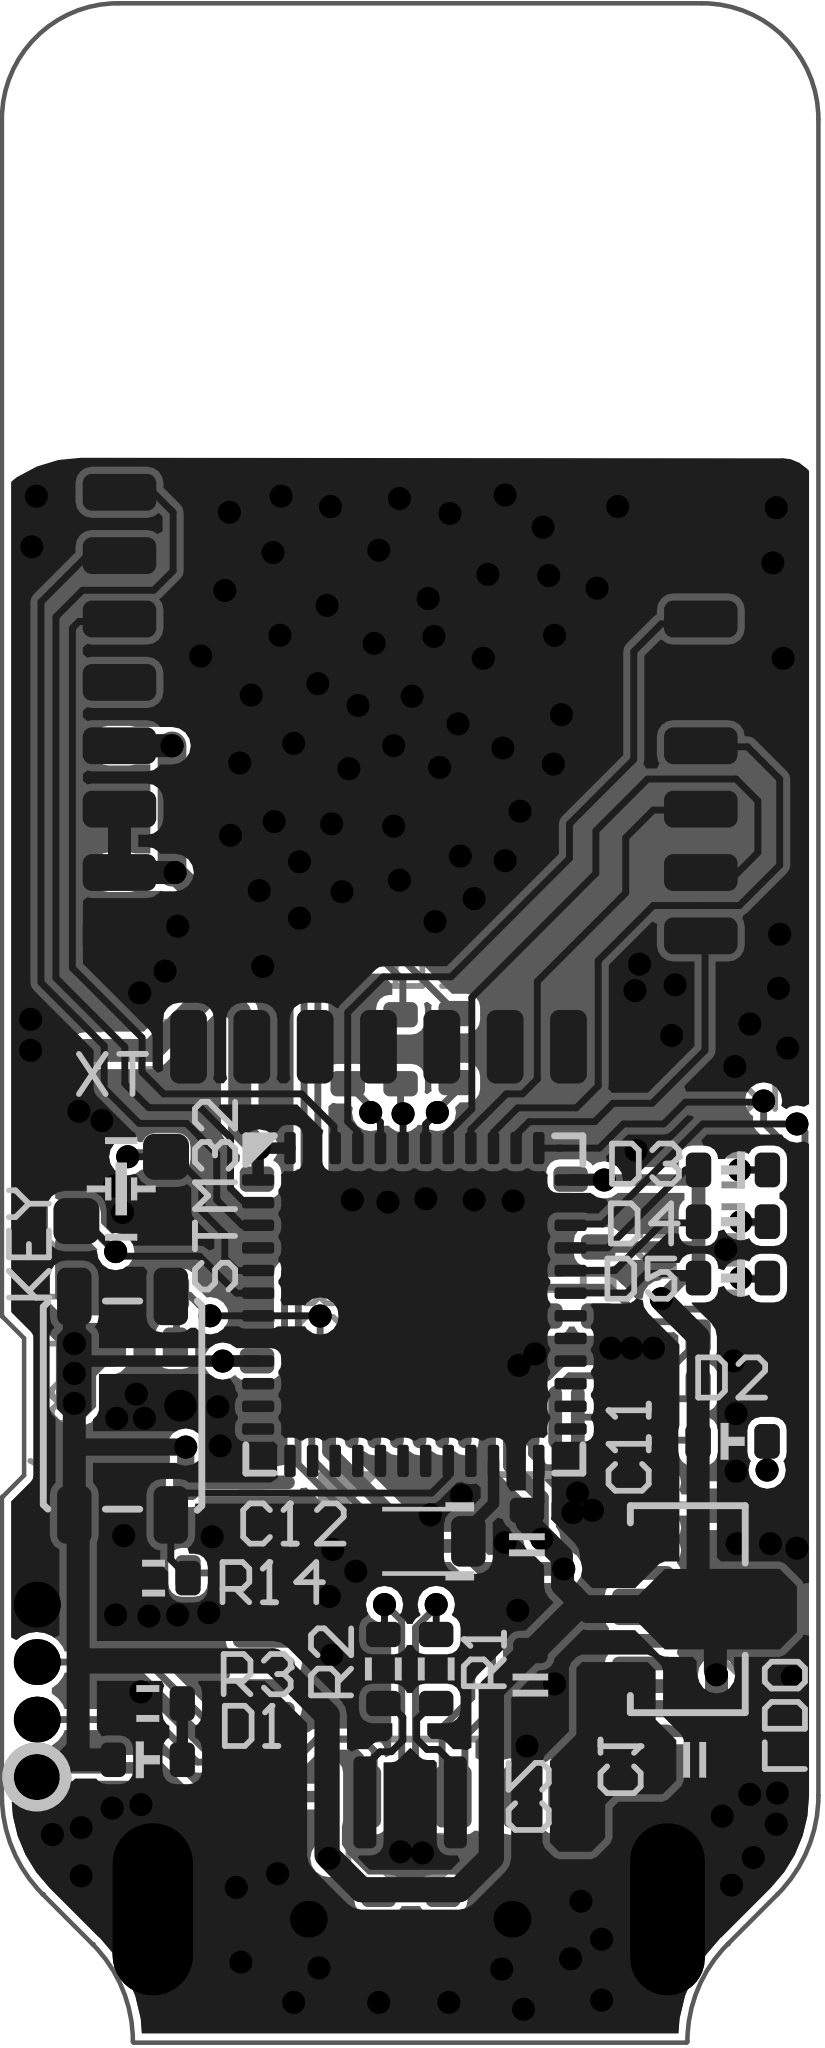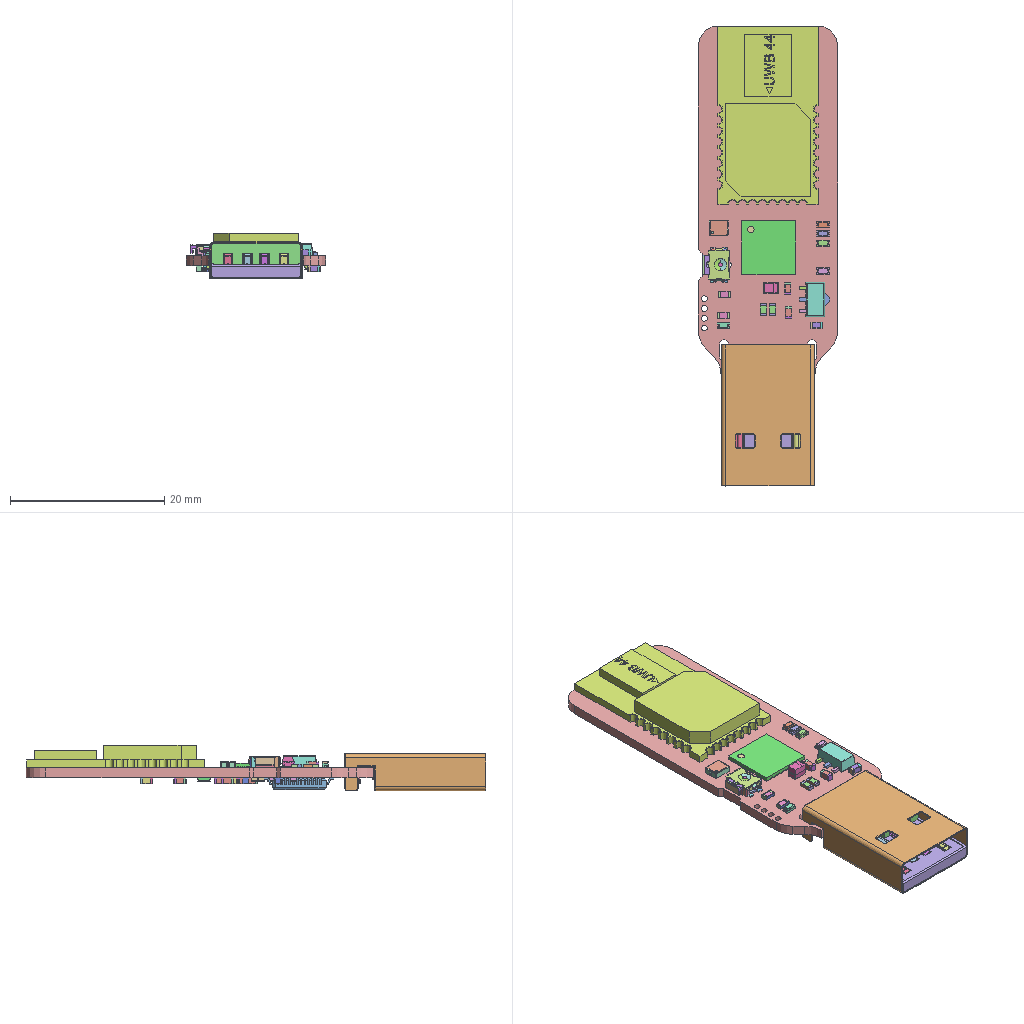Circuit board layout | Altium Designer | box 18.1 x 59.7 x 5.9 mm
Layer stack:
# Altium Designer layer stack of 9 (unit mm; dielectric type: 0 none, 1 core, 2 prepreg, 3 surface material)
index,name,kind,layer,copper_thickness_mm,dielectric_type,dielectric_thickness_mm,dielectric_material,dielectric_constant
0,Top Paste,other,,,,,,
1,Top Overlay,other,,,,,,
2,Top Solder,dielectric,,,3,0.01,Solder Resist,3.5
3,Top Layer,copper,Top Layer,0.03,,,,
4,Dielectric1,dielectric,,,1,1.2,,4.2
5,Bottom Layer,copper,Bottom Layer,0.03,,,,
6,Bottom Solder,dielectric,,,3,0.01,Solder Resist,3.5
7,Bottom Overlay,other,,,,,,
8,Bottom Paste,other,,,,,,
# drill layer pairs: low layer,high layer
drill_pair,Top Layer,Bottom Layer
Part placement:
Designator,Comment,Layer,Footprint,Center-X(mm),Center-Y(mm),Rotation
LDO,AMS1117,TopLayer,SOT89-3,10.617,9.55,360
USB,USB_Plug_TypeA,TopLayer,USB_Plug_TypeA,6.104,3.992,270
XT,XTAL_2520_4P,TopLayer,XT_2520_4,-0.2837,18.834,360
R14,Res_0603,TopLayer,RES_0603,0.4318,10.236,360
R13,Res_0603,BottomLayer,RES_0603,0.1524,15.392,180
R12,Res_0603,BottomLayer,RES_0603,4.724,21.92,90
R11,Res_0603,BottomLayer,RES_0603,7.112,21.946,90
R10,Res_0603,BottomLayer,RES_0603,5.893,21.92,90
R9,Res_0603,BottomLayer,RES_0603,13.614,11.836,180
R8,Res_0603,BottomLayer,RES_0603,13.233,14.453,180
R7,Res_0603,BottomLayer,RES_0603,13.233,15.57,180
R6,Res_0603,BottomLayer,RES_0603,0.4318,10.363,360
R5,Res_0603,BottomLayer,RES_0603,10.262,16.789,90
R4,Res_0603,BottomLayer,RES_0603,13.233,13.259,360
R3,Res_0603,TopLayer,RES_0603,0.3048,7.468,360
R2,Res_0603,TopLayer,RES_0603,5.512,8.23,90
R1,Res_0603,TopLayer,RES_0603,6.68,8.23,90
KEY,ButtonTACT,TopLayer,ButtonTACT_3.5*3.55_90,-0.1524,14.046,90
C17,Cap_0603,BottomLayer,CAP_0603,-0.3302,29.388,90
C16,Cap_0603,BottomLayer,CAP_0603,-0.3302,25.07,270
C13,Cap_0603,BottomLayer,CAP_0603,0.1778,16.535,360
C11,Cap_0603,TopLayer,CAP_0603,8.687,10.973,90
C10,Cap_0603,BottomLayer,CAP_0603,9.652,19.812,270
C9,Cap_0603,BottomLayer,CAP_0603,2.718,18.288,90
C8,Cap_0603,BottomLayer,CAP_0603,2.718,15.799,270
C7,Cap_0603,BottomLayer,CAP_0603,13.64,6.858,180
C6,Cap_0603,BottomLayer,CAP_0603,0.381,12.344,360
C5,Cap_0603,BottomLayer,CAP_0603,6.833,2.489,90
C4,Cap_0603,BottomLayer,CAP_0603,5.41,2.489,90
C3,Cap_0603,BottomLayer,CAP_0603,9.093,16.789,270
STM32,STM32F411C,TopLayer,QFN_P0.5_48,6.198,16.281,360
STM32J,STM32F072C,BottomLayer,LQFP_P0.5_48,7.061,9.601,270
DWM,DWM1000,TopLayer,DWM1000,6.104,28.099,0
D2,LED_0603,TopLayer,LED_0603_ORANGE,13.233,13.259,360
D1,LED_0603,TopLayer,LED_0603_YELLOW,0.3048,6.223,360
C1,Cap_0603,TopLayer,CAP_0603,12.395,6.223,180
C2,Cap_0603,TopLayer,CAP_0603,8.763,7.874,90
D3,LED_0603,TopLayer,LED_0603_RED,13.242,19.253,180
D4,LED_0603,TopLayer,LED_0603_GREEN,13.242,18.11,180
D5,LED_0603,TopLayer,LED_0603_BLUE,13.242,16.866,180
R15,Res_0603,BottomLayer,RES_0603,13.242,19.253,180
R16,Res_0603,BottomLayer,RES_0603,13.242,18.11,180
R17,Res_0603,BottomLayer,RES_0603,13.242,16.866,180
C12,Cap_Tan_0805,TopLayer,CAP_TAN_P0805,6.502,11.049,180
C15,Cap_0603,BottomLayer,CAP_0603,-1.27,18.923,270
C14,Cap_0603,BottomLayer,CAP_0603,0.7112,18.872,90
Pad and via stacks:
# Altium Designer via and pad stacks of 9 (unit mm). Each distinct definition once, with the count of objects using it.
# via: kind,start_layer,end_layer,hole_mm,diameter_mm,mode(0 simple;1 top-mid-bottom;2 full stack),diameter_per_layer,count,example_net
# pad: kind,layer,hole_mm,hole_type(0 round;1 square;2 slot),plating,top_size,top_shape(1 round;2 rect;3 octagon;9 rounded rect),mid_size,bottom_size,mode,footprint,size_per_layer,count,example
pad,Top Layer,0,0,plated,0.762x0.5588,9,0.762x0.5588,0.762x0.5588,0,RES_0603,,8,R3.2
pad,Top Layer,0,0,plated,1.118x0.762,9,1.118x0.762,1.118x0.762,0,CAP_TAN_P0805,,2,C12.1
pad,Top Layer,0,0,plated,0.762x0.5588,9,0.762x0.5588,0.762x0.5588,0,LED_0603_BLUE,,2,D5.1
pad,Top Layer,0,0,plated,0.762x0.5588,9,0.762x0.5588,0.762x0.5588,0,LED_0603_GREEN,,2,D4.2
pad,Top Layer,0,0,plated,0.762x0.5588,9,0.762x0.5588,0.762x0.5588,0,LED_0603_RED,,2,D3.1
pad,Top Layer,0,0,plated,0.762x0.5588,9,0.762x0.5588,0.762x0.5588,0,LED_0603_YELLOW,,2,D1.1
pad,Top Layer,0,0,plated,0.762x0.5588,9,0.762x0.5588,0.762x0.5588,0,LED_0603_ORANGE,,2,D2.2
pad,Top Layer,0,0,plated,0.254x0.7112,9,0.254x0.7112,0.254x0.7112,0,QFN_P0.5_48,,48,STM32.47
pad,Top Layer,0,0,plated,3.353x3.353,9,3.353x3.353,3.353x3.353,0,QFN_P0.5_48,,1,STM32.49
pad,Top Layer,0,0,plated,1.27x0.762,9,1.27x0.762,1.27x0.762,0,ButtonTACT_3.5*3.55_90,,4,KEY.3
pad,Top Layer,0,0,plated,1.016x1.016,9,1.016x1.016,1.016x1.016,0,XT_2520_4,,4,XT.1
pad,Top Layer,0,0,plated,0.508x2.032,9,0.508x2.032,0.508x2.032,0,USB_Plug_TypeA,,4,USB.1
pad,Top Layer,0,0,plated,0.8128x1.626,9,0.8128x1.626,0.8128x1.626,0,DWM1000,,24,DWM.15
pad,Top Layer,0,0,plated,0.762x0.5588,9,0.762x0.5588,0.762x0.5588,0,CAP_0603,,6,C1.2
pad,Top Layer,0,0,plated,0.5588x1.524,9,0.5588x1.524,0.5588x1.524,0,SOT89-3,,2,LDO.1
pad,Top Layer,0,0,plated,0.6096x1.524,9,0.6096x1.524,0.6096x1.524,0,SOT89-3,,1,LDO.2
pad,Multi-Layer,0.7,0,plated,0.7x0.7,1,0.7x0.7,0.7x0.7,0,ButtonTACT_3.5*3.55_90,,1,KEY.0
pad,Multi-Layer,1.143,2,plated,1.778x3.81,1,1.778x3.81,1.778x3.81,0,USB_Plug_TypeA,,1,USB.4
pad,Multi-Layer,1.067,0,plated,0.8128x0.8128,1,0.8128x0.8128,0.8128x0.8128,0,USB_Plug_TypeA,,2,USB.0
pad,Multi-Layer,1.143,2,plated,1.651x3.81,1,1.651x3.81,1.651x3.81,0,USB_Plug_TypeA,,1,USB.4
pad,Multi-Layer,0.762,0,plated,1.016x1.016,1,1.016x1.016,1.016x1.016,0,,,4,1
pad,Bottom Layer,0,0,plated,0.762x0.5588,9,0.762x0.5588,0.762x0.5588,0,RES_0603,,26,R5.2
pad,Bottom Layer,0,0,plated,0.3048x1.372,1,0.3048x1.372,0.3048x1.372,0,LQFP_P0.5_48,,48,STM32J.46
pad,Bottom Layer,0,0,plated,0.762x0.5588,9,0.762x0.5588,0.762x0.5588,0,CAP_0603,,26,C3.2
via,Top Layer,Bottom Layer,0.3048,0.508,0,,188,GND
Copper pours:
name,layer,net,type(0 solid;1 hatched;2 none)
Top Layer-No Net,Top Layer,GND,0
Top Layer-No Net,Top Layer,3V3,0
Top Layer-No Net,Top Layer,VUSB,0
Top Layer-No Net,Bottom Layer,GND,0
Top Layer-No Net,Bottom Layer,3V3,0
Design rules, without the lines most boards share:
# Altium Designer design rules of 9 (exported by Altium Designer, unit mm)
# columns: name | kind | enabled | priority | scope1 | scope2 | descriptor | typed fields (field=value)
Clearance | 0 | enabled | 1 | All | All | Clearance Constraint (Gap=6mil) (All),(All) | gap=0.1524
PlaneConnect | 6 | enabled | 1 | All | All | Power Plane Connect Rule(Relief Connect )(Expansion=20mil) (Conductor Width=10mil) (Air Gap=10mil) (Entries=4) (All) | relief_conductor_width=0.254 relief_entries=4 relief_expansion=0.508
PolygonConnect | 20 | enabled | 1 | All | All | Polygon Connect Rule(Direct Connect )(Conductor Width=10mil) (Relief Angle=90 Angle) (Entries=4) (Air Gap Width=10mil) (All),(All) | connect_style(0=relief,1=direct,2=none)=1 relief_conductor_width=0.254 relief_entries=4
Width | 2 | enabled | 1 | All | All | Width Constraint (Min=6mil) (Max=50mil) (Preferred=10mil) (All) |
RoutingVias | 11 | enabled | 1 | All | All | Routing Via (MinHoleWidth=12mil) (MaxHoleWidth=12mil) (PreferredHoleWidth=12mil) (MinWidth=20mil) (MaxWidth=20mil) (PreferedWidth=20mil) (All) | via_min_hole=0.3048 via_max_hole=0.3048 via_preferred_diameter=0.508 via_preferred_hole=0.3048
PasteMaskExpansion | 14 | enabled | 1 | All | All | Paste Mask Expansion (Expansion =0mil) (All) | expansion=0
SolderMaskExpansion | 13 | enabled | 1 | All | All | Solder Mask Expansion (Expansion =2mil) (All) | expansion=0.0508
ComponentClearance | 24 | enabled | 1 | All | All | Component Clearance Constraint ( Horizontal Gap = 0mil, Vertical Gap = 0mil ) (All),(All)  | gap=0
Height | 50 | enabled | 1 | All | All | Height Constraint (Min=0mil) (Max=5000mil) (Prefered=500mil) (All) | min_height=0 max_height=127
HoleSize | 42 | enabled | 1 | All | All | Hole Size Constraint (Min=1mil) (Max=200mil) (All) |
DiffPairsRouting | 51 | enabled | 1 | All | All | Differential Pairs Uncoupled Length using the Gap Constraints (Min=10mil) (Max=10mil) (Prefered=10mil)  and Width Constraints (Min=15mil) (Max=15mil) (Prefered=15mil) (All) |
HoleToHoleClearance | 52 | enabled | 1 | All | All | Hole To Hole Clearance (Gap=0mil) (All),(All) | gap=0
MinimumSolderMaskSliver | 53 | enabled | 1 | All | All | Minimum Solder Mask Sliver (Gap=0mil) (All),(All) |
SilkToSolderMaskClearance | 54 | enabled | 1 | IsPad | All | Silk To Solder Mask (Clearance=0mil) (IsPad),(All) |
SilkToSilkClearance | 55 | enabled | 1 | All | All | Silk to Silk (Clearance=0mil) (All),(All) |
Classes set for this board:
# Altium Designer classes of 9 (member kind: 0 net, 1 component, 2 from-to, 3 pad, 4 layer, 5 differential pair, 6 design channel, 7 polygon, 8 structure, 9 xSignal)
# columns: class name | member kind | superclass | members
UWB-Adapter_Sch | 1 | no | D1; D2; STM32; C3; C4; C5; C6; C7; C8; C9; C10; C11; C13; C16; C17; KEY; R1; R2; R3; R4; R5; R6; R7; R8; R9; R10; R11; R12; R13; R14; XT; STM32J; C1; C2; D3; D4; D5; DWM; C12; C14; C15; LDO; USB; R17; R16; R15;